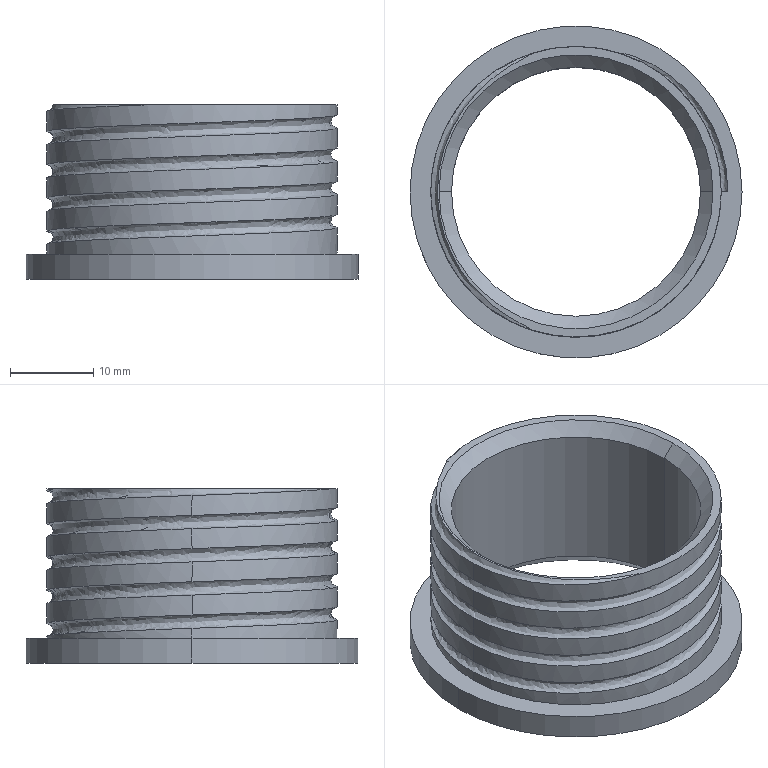Part | NX | features SKETCH 3, DATUM_CSYS 2, BREP 1, CHAMFER 1, DATUM_ON_PATH 1, EXTRUDE 1, HELIX 1, VARIATIONAL_SWEEP 1 | 1 solid | 24 faces | volume 5444 mm3 | cylinder 15 | cone 4 | plane 4 | spline 1 | commonest cylinder face diameters 35 x11 30 x2 40 x2